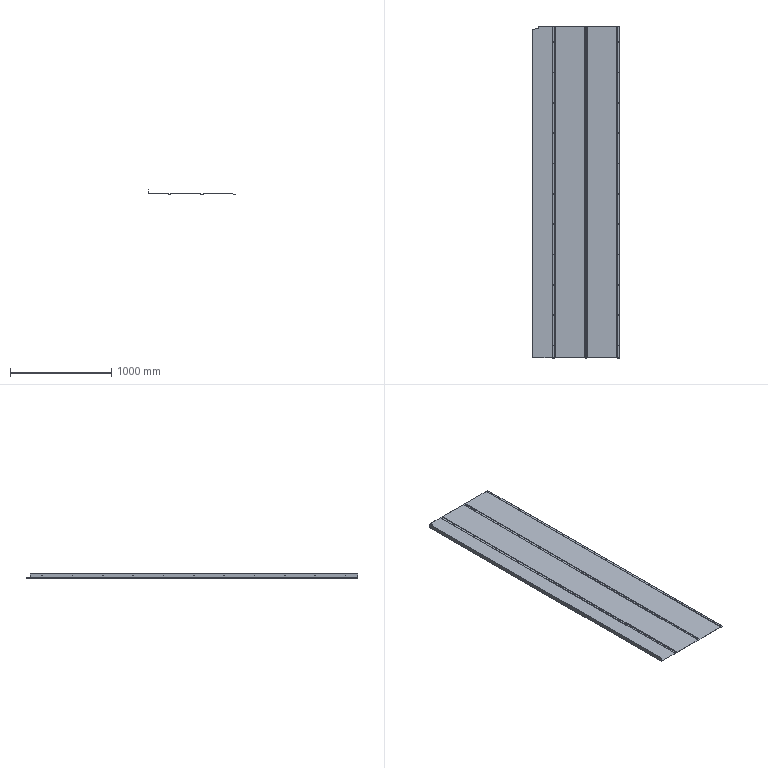Part | STEP file | TS-S101 | 1 solid | 189 faces | box 859 x 3283 x 43 mm | volume 3553710 mm3 | cylinder 113 | plane 76 | commonest cylinder face diameters 5.4 x88 0.4 x11 2.8 x11 10 x1 16 x1 18 x1